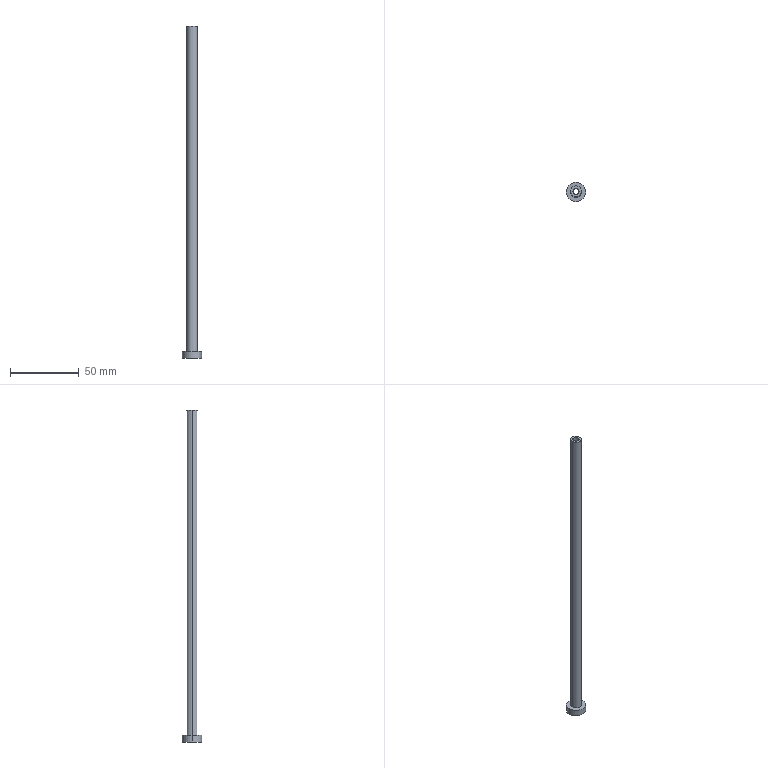Part | Creo | 1 solid | 9 faces | box 14 x 14 x 242.236 mm | volume 8842 mm3 | cylinder 6 | plane 3 | commonest cylinder face diameters 4.5 x2 8 x2 14 x2
STEP:
#1=CARTESIAN_POINT('',(-180.234,-210.84,6.736));
#2=VERTEX_POINT('',#1);
#3=CARTESIAN_POINT('',(-188.234,-210.84,6.736));
#4=VERTEX_POINT('',#3);
#5=CARTESIAN_POINT('',(-184.234,-210.84,6.736));
#6=DIRECTION('',(0.,0.,1.));
#7=DIRECTION('',(1.,0.,0.));
#8=AXIS2_PLACEMENT_3D('',#5,#6,#7);
#9=CIRCLE('',#8,4.);
#10=EDGE_CURVE('',#2,#4,#9,.T.);
#11=ORIENTED_EDGE('',*,*,#10,.F.);
#12=CARTESIAN_POINT('',(-184.234,-210.84,6.736));
#13=DIRECTION('',(0.,0.,1.));
#14=DIRECTION('',(-1.,0.,0.));
#15=AXIS2_PLACEMENT_3D('',#12,#13,#14);
#16=CIRCLE('',#15,4.);
#17=EDGE_CURVE('',#4,#2,#16,.T.);
#18=ORIENTED_EDGE('',*,*,#17,.F.);
#19=EDGE_LOOP('',(#11,#18));
#20=FACE_OUTER_BOUND('',#19,.F.);
#21=CARTESIAN_POINT('',(-181.984,-210.84,6.736));
#22=VERTEX_POINT('',#21);
#23=CARTESIAN_POINT('',(-186.484,-210.84,6.736));
#24=VERTEX_POINT('',#23);
#25=CARTESIAN_POINT('',(-184.234,-210.84,6.736));
#26=DIRECTION('',(0.,0.,-1.));
#27=DIRECTION('',(1.,0.,0.));
#28=AXIS2_PLACEMENT_3D('',#25,#26,#27);
#29=CIRCLE('',#28,2.25);
#30=EDGE_CURVE('',#22,#24,#29,.T.);
#31=ORIENTED_EDGE('',*,*,#30,.F.);
#32=CARTESIAN_POINT('',(-184.234,-210.84,6.736));
#33=DIRECTION('',(0.,0.,-1.));
#34=DIRECTION('',(-1.,0.,0.));
#35=AXIS2_PLACEMENT_3D('',#32,#33,#34);
#36=CIRCLE('',#35,2.25);
#37=EDGE_CURVE('',#24,#22,#36,.T.);
#38=ORIENTED_EDGE('',*,*,#37,.F.);
#39=EDGE_LOOP('',(#31,#38));
#40=FACE_BOUND('',#39,.F.);
#41=CARTESIAN_POINT('',(-1.827,-11.85,6.736));
#42=DIRECTION('',(0.,0.,1.));
#43=DIRECTION('',(0.,-1.,0.));
#44=AXIS2_PLACEMENT_3D('',#41,#42,#43);
#45=PLANE('',#44);
#46=ADVANCED_FACE('',(#20,#40),#45,.T.);
#47=CARTESIAN_POINT('',(-188.234,-210.84,-230.5));
#48=VERTEX_POINT('',#47);
#49=CARTESIAN_POINT('',(-180.234,-210.84,-230.5));
#50=VERTEX_POINT('',#49);
#51=CARTESIAN_POINT('',(-184.234,-210.84,-230.5));
#52=DIRECTION('',(0.,0.,-1.));
#53=DIRECTION('',(-1.,0.,0.));
#54=AXIS2_PLACEMENT_3D('',#51,#52,#53);
#55=CIRCLE('',#54,4.);
#56=EDGE_CURVE('',#48,#50,#55,.T.);
#57=ORIENTED_EDGE('',*,*,#56,.T.);
#58=CARTESIAN_POINT('',(-180.234,-210.84,6.736));
#59=DIRECTION('',(0.,0.,-1.));
#60=VECTOR('',#59,237.236);
#61=LINE('',#58,#60);
#62=EDGE_CURVE('',#2,#50,#61,.T.);
#63=ORIENTED_EDGE('',*,*,#62,.F.);
#64=ORIENTED_EDGE('',*,*,#10,.T.);
#65=CARTESIAN_POINT('',(-188.234,-210.84,6.736));
#66=DIRECTION('',(0.,0.,-1.));
#67=VECTOR('',#66,237.236);
#68=LINE('',#65,#67);
#69=EDGE_CURVE('',#4,#48,#68,.T.);
#70=ORIENTED_EDGE('',*,*,#69,.T.);
#71=EDGE_LOOP('',(#57,#63,#64,#70));
#72=FACE_OUTER_BOUND('',#71,.F.);
#73=CARTESIAN_POINT('',(-184.234,-210.84,7.391));
#74=DIRECTION('',(0.,0.,-1.));
#75=DIRECTION('',(1.,0.,0.));
#76=AXIS2_PLACEMENT_3D('',#73,#74,#75);
#77=CYLINDRICAL_SURFACE('',#76,4.);
#78=ADVANCED_FACE('',(#72),#77,.T.);
#79=CARTESIAN_POINT('',(-177.234,-210.84,-230.5));
#80=VERTEX_POINT('',#79);
#81=CARTESIAN_POINT('',(-191.234,-210.84,-230.5));
#82=VERTEX_POINT('',#81);
#83=CARTESIAN_POINT('',(-184.234,-210.84,-230.5));
#84=DIRECTION('',(0.,0.,1.));
#85=DIRECTION('',(1.,0.,0.));
#86=AXIS2_PLACEMENT_3D('',#83,#84,#85);
#87=CIRCLE('',#86,7.);
#88=EDGE_CURVE('',#80,#82,#87,.T.);
#89=ORIENTED_EDGE('',*,*,#88,.F.);
#90=CARTESIAN_POINT('',(-184.234,-210.84,-230.5));
#91=DIRECTION('',(0.,0.,1.));
#92=DIRECTION('',(-1.,0.,0.));
#93=AXIS2_PLACEMENT_3D('',#90,#91,#92);
#94=CIRCLE('',#93,7.);
#95=EDGE_CURVE('',#82,#80,#94,.T.);
#96=ORIENTED_EDGE('',*,*,#95,.F.);
#97=EDGE_LOOP('',(#89,#96));
#98=FACE_OUTER_BOUND('',#97,.F.);
#99=CARTESIAN_POINT('',(-184.234,-210.84,-230.5));
#100=DIRECTION('',(0.,0.,-1.));
#101=DIRECTION('',(1.,0.,0.));
#102=AXIS2_PLACEMENT_3D('',#99,#100,#101);
#103=CIRCLE('',#102,4.);
#104=EDGE_CURVE('',#50,#48,#103,.T.);
#105=ORIENTED_EDGE('',*,*,#104,.F.);
#106=ORIENTED_EDGE('',*,*,#56,.F.);
#107=EDGE_LOOP('',(#105,#106));
#108=FACE_BOUND('',#107,.F.);
#109=CARTESIAN_POINT('',(-184.234,-210.84,-230.5));
#110=DIRECTION('',(0.,0.,1.));
#111=DIRECTION('',(-1.,0.,0.));
#112=AXIS2_PLACEMENT_3D('',#109,#110,#111);
#113=PLANE('',#112);
#114=ADVANCED_FACE('',(#98,#108),#113,.T.);
#115=ORIENTED_EDGE('',*,*,#104,.T.);
#116=ORIENTED_EDGE('',*,*,#69,.F.);
#117=ORIENTED_EDGE('',*,*,#17,.T.);
#118=ORIENTED_EDGE('',*,*,#62,.T.);
#119=EDGE_LOOP('',(#115,#116,#117,#118));
#120=FACE_OUTER_BOUND('',#119,.F.);
#121=CARTESIAN_POINT('',(-184.234,-210.84,7.391));
#122=DIRECTION('',(0.,0.,-1.));
#123=DIRECTION('',(1.,0.,0.));
#124=AXIS2_PLACEMENT_3D('',#121,#122,#123);
#125=CYLINDRICAL_SURFACE('',#124,4.);
#126=ADVANCED_FACE('',(#120),#125,.T.);
#127=ORIENTED_EDGE('',*,*,#88,.T.);
#128=CARTESIAN_POINT('',(-191.234,-210.84,-235.5));
#129=VERTEX_POINT('',#128);
#130=CARTESIAN_POINT('',(-191.234,-210.84,-235.5));
#131=DIRECTION('',(0.,0.,1.));
#132=VECTOR('',#131,5.);
#133=LINE('',#130,#132);
#134=EDGE_CURVE('',#129,#82,#133,.T.);
#135=ORIENTED_EDGE('',*,*,#134,.F.);
#136=CARTESIAN_POINT('',(-177.234,-210.84,-235.5));
#137=VERTEX_POINT('',#136);
#138=CARTESIAN_POINT('',(-184.234,-210.84,-235.5));
#139=DIRECTION('',(0.,0.,-1.));
#140=DIRECTION('',(-1.,0.,0.));
#141=AXIS2_PLACEMENT_3D('',#138,#139,#140);
#142=CIRCLE('',#141,7.);
#143=EDGE_CURVE('',#129,#137,#142,.T.);
#144=ORIENTED_EDGE('',*,*,#143,.T.);
#145=CARTESIAN_POINT('',(-177.234,-210.84,-235.5));
#146=DIRECTION('',(0.,0.,1.));
#147=VECTOR('',#146,5.);
#148=LINE('',#145,#147);
#149=EDGE_CURVE('',#137,#80,#148,.T.);
#150=ORIENTED_EDGE('',*,*,#149,.T.);
#151=EDGE_LOOP('',(#127,#135,#144,#150));
#152=FACE_OUTER_BOUND('',#151,.F.);
#153=CARTESIAN_POINT('',(-184.234,-210.84,-235.5));
#154=DIRECTION('',(0.,0.,1.));
#155=DIRECTION('',(-1.,0.,0.));
#156=AXIS2_PLACEMENT_3D('',#153,#154,#155);
#157=CYLINDRICAL_SURFACE('',#156,7.);
#158=ADVANCED_FACE('',(#152),#157,.T.);
#159=ORIENTED_EDGE('',*,*,#95,.T.);
#160=ORIENTED_EDGE('',*,*,#149,.F.);
#161=CARTESIAN_POINT('',(-184.234,-210.84,-235.5));
#162=DIRECTION('',(0.,0.,-1.));
#163=DIRECTION('',(1.,0.,0.));
#164=AXIS2_PLACEMENT_3D('',#161,#162,#163);
#165=CIRCLE('',#164,7.);
#166=EDGE_CURVE('',#137,#129,#165,.T.);
#167=ORIENTED_EDGE('',*,*,#166,.T.);
#168=ORIENTED_EDGE('',*,*,#134,.T.);
#169=EDGE_LOOP('',(#159,#160,#167,#168));
#170=FACE_OUTER_BOUND('',#169,.F.);
#171=CARTESIAN_POINT('',(-184.234,-210.84,-235.5));
#172=DIRECTION('',(0.,0.,1.));
#173=DIRECTION('',(-1.,0.,0.));
#174=AXIS2_PLACEMENT_3D('',#171,#172,#173);
#175=CYLINDRICAL_SURFACE('',#174,7.);
#176=ADVANCED_FACE('',(#170),#175,.T.);
#177=ORIENTED_EDGE('',*,*,#143,.F.);
#178=ORIENTED_EDGE('',*,*,#166,.F.);
#179=EDGE_LOOP('',(#177,#178));
#180=FACE_OUTER_BOUND('',#179,.F.);
#181=CARTESIAN_POINT('',(-181.984,-210.84,-235.5));
#182=VERTEX_POINT('',#181);
#183=CARTESIAN_POINT('',(-186.484,-210.84,-235.5));
#184=VERTEX_POINT('',#183);
#185=CARTESIAN_POINT('',(-184.234,-210.84,-235.5));
#186=DIRECTION('',(0.,0.,1.));
#187=DIRECTION('',(1.,0.,0.));
#188=AXIS2_PLACEMENT_3D('',#185,#186,#187);
#189=CIRCLE('',#188,2.25);
#190=EDGE_CURVE('',#182,#184,#189,.T.);
#191=ORIENTED_EDGE('',*,*,#190,.F.);
#192=CARTESIAN_POINT('',(-184.234,-210.84,-235.5));
#193=DIRECTION('',(0.,0.,1.));
#194=DIRECTION('',(-1.,0.,0.));
#195=AXIS2_PLACEMENT_3D('',#192,#193,#194);
#196=CIRCLE('',#195,2.25);
#197=EDGE_CURVE('',#184,#182,#196,.T.);
#198=ORIENTED_EDGE('',*,*,#197,.F.);
#199=EDGE_LOOP('',(#191,#198));
#200=FACE_BOUND('',#199,.F.);
#201=CARTESIAN_POINT('',(-246.549,-847.518,-235.5));
#202=DIRECTION('',(0.,0.,-1.));
#203=DIRECTION('',(1.,0.,0.));
#204=AXIS2_PLACEMENT_3D('',#201,#202,#203);
#205=PLANE('',#204);
#206=ADVANCED_FACE('',(#180,#200),#205,.T.);
#207=ORIENTED_EDGE('',*,*,#190,.T.);
#208=CARTESIAN_POINT('',(-186.484,-210.84,6.736));
#209=DIRECTION('',(0.,0.,-1.));
#210=VECTOR('',#209,242.236);
#211=LINE('',#208,#210);
#212=EDGE_CURVE('',#24,#184,#211,.T.);
#213=ORIENTED_EDGE('',*,*,#212,.F.);
#214=ORIENTED_EDGE('',*,*,#37,.T.);
#215=CARTESIAN_POINT('',(-181.984,-210.84,6.736));
#216=DIRECTION('',(0.,0.,-1.));
#217=VECTOR('',#216,242.236);
#218=LINE('',#215,#217);
#219=EDGE_CURVE('',#22,#182,#218,.T.);
#220=ORIENTED_EDGE('',*,*,#219,.T.);
#221=EDGE_LOOP('',(#207,#213,#214,#220));
#222=FACE_OUTER_BOUND('',#221,.F.);
#223=CARTESIAN_POINT('',(-184.234,-210.84,7.391));
#224=DIRECTION('',(0.,0.,-1.));
#225=DIRECTION('',(1.,0.,0.));
#226=AXIS2_PLACEMENT_3D('',#223,#224,#225);
#227=CYLINDRICAL_SURFACE('',#226,2.25);
#228=ADVANCED_FACE('',(#222),#227,.F.);
#229=ORIENTED_EDGE('',*,*,#197,.T.);
#230=ORIENTED_EDGE('',*,*,#219,.F.);
#231=ORIENTED_EDGE('',*,*,#30,.T.);
#232=ORIENTED_EDGE('',*,*,#212,.T.);
#233=EDGE_LOOP('',(#229,#230,#231,#232));
#234=FACE_OUTER_BOUND('',#233,.F.);
#235=CARTESIAN_POINT('',(-184.234,-210.84,7.391));
#236=DIRECTION('',(0.,0.,-1.));
#237=DIRECTION('',(1.,0.,0.));
#238=AXIS2_PLACEMENT_3D('',#235,#236,#237);
#239=CYLINDRICAL_SURFACE('',#238,2.25);
#240=ADVANCED_FACE('',(#234),#239,.F.);
#241=CLOSED_SHELL('',(#46,#78,#114,#126,#158,#176,#206,#228,#240));
#242=MANIFOLD_SOLID_BREP('',#241);
#243=(LENGTH_UNIT()NAMED_UNIT(*)SI_UNIT(.MILLI.,.METRE.));
#244=UNCERTAINTY_MEASURE_WITH_UNIT(LENGTH_MEASURE(0.0243),#243,'','');
#245=(NAMED_UNIT(*)PLANE_ANGLE_UNIT()SI_UNIT($,.RADIAN.));
#246=PLANE_ANGLE_MEASURE_WITH_UNIT(PLANE_ANGLE_MEASURE(0.01745),#245);
#247=(CONVERSION_BASED_UNIT('DEGREE',#246)NAMED_UNIT(*)PLANE_ANGLE_UNIT());
#248=(NAMED_UNIT(*)SI_UNIT($,.STERADIAN.)SOLID_ANGLE_UNIT());
#249=(GEOMETRIC_REPRESENTATION_CONTEXT(3)GLOBAL_UNCERTAINTY_ASSIGNED_CONTEXT((#244))GLOBAL_UNIT_ASSIGNED_CONTEXT((#243,#247,#248))REPRESENTATION_CONTEXT('',''));
#250=ADVANCED_BREP_SHAPE_REPRESENTATION('',(#242),#249);